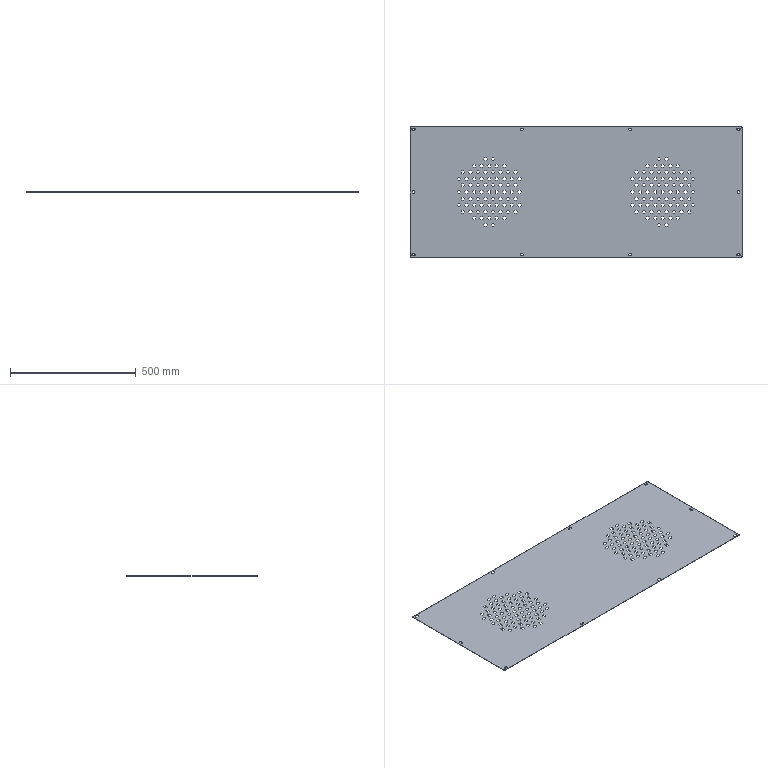Part | SolidWorks | features BaseBody 1 | 1 solid | 934 faces | box 1320 x 520 x 1.2 mm | volume 800672 mm3 | plane 902 | cylinder 32 | commonest cylinder face diameters 7 x28 10 x4